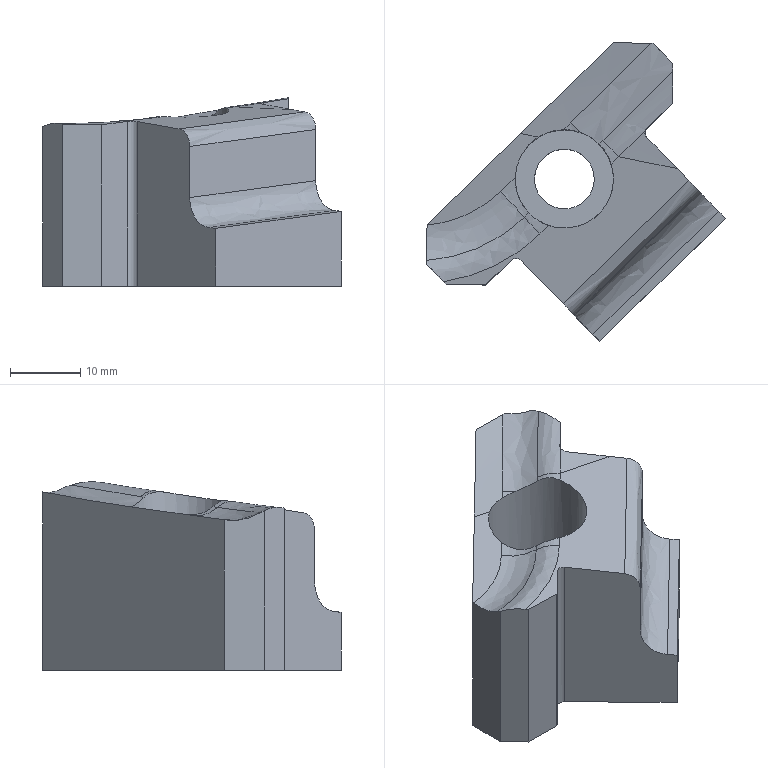Part | STEP file | gslz 2016.10.28-13_id1626_x_t | 1 solid | 34 faces | box 42.516 x 42.404 x 26.831 mm | volume 17674 mm3 | plane 15 | spline 15 | cylinder 4 | commonest cylinder face diameters 2 x2 8.5 x1 14 x1